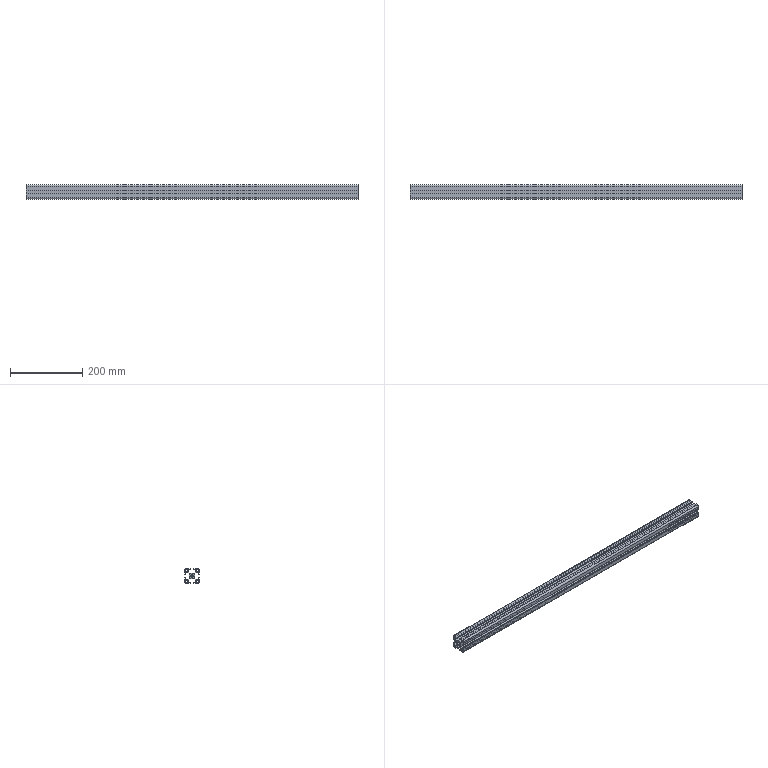Part | SolidWorks | features WeldMemberFeat 1, WeldmentFeature 1 | 1 solid | 104 faces | box 920 x 40 x 40 mm | volume 530422 mm3 | plane 94 | cylinder 10 | commonest cylinder face diameters 5 x4 9 x4 6.8 x2